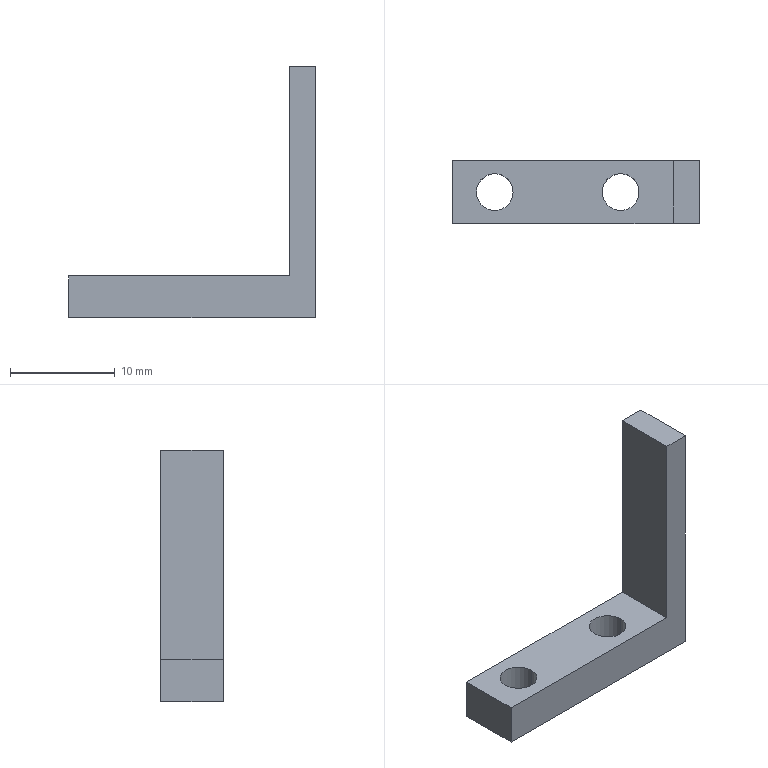Part | SolidWorks | features BaseBody 1 | 1 solid | 12 faces | box 23.5 x 6 x 24 mm | volume 787.031 mm3 | plane 8 | cylinder 4 | commonest cylinder face diameters 3.5 x4
STEP:
#1=CARTESIAN_POINT('',(-33.678,3.,0.));
#2=VERTEX_POINT('',#1);
#3=CARTESIAN_POINT('',(-37.178,3.,0.));
#4=VERTEX_POINT('',#3);
#5=CARTESIAN_POINT('',(-35.428,3.,0.));
#6=DIRECTION('',(0.,0.,-1.));
#7=DIRECTION('',(1.,0.,0.));
#8=AXIS2_PLACEMENT_3D('',#5,#6,#7);
#9=CIRCLE('',#8,1.75);
#10=EDGE_CURVE('',#2,#4,#9,.T.);
#11=ORIENTED_EDGE('',*,*,#10,.T.);
#12=CARTESIAN_POINT('',(-37.178,3.,4.));
#13=VERTEX_POINT('',#12);
#14=CARTESIAN_POINT('',(-37.178,3.,-30.121));
#15=DIRECTION('',(0.,0.,1.));
#16=VECTOR('',#15,1000.);
#17=LINE('',#14,#16);
#18=EDGE_CURVE('',#4,#13,#17,.T.);
#19=ORIENTED_EDGE('',*,*,#18,.T.);
#20=CARTESIAN_POINT('',(-33.678,3.,4.));
#21=VERTEX_POINT('',#20);
#22=CARTESIAN_POINT('',(-35.428,3.,4.));
#23=DIRECTION('',(0.,0.,-1.));
#24=DIRECTION('',(1.,0.,0.));
#25=AXIS2_PLACEMENT_3D('',#22,#23,#24);
#26=CIRCLE('',#25,1.75);
#27=EDGE_CURVE('',#21,#13,#26,.T.);
#28=ORIENTED_EDGE('',*,*,#27,.F.);
#29=CARTESIAN_POINT('',(-33.678,3.,-30.121));
#30=DIRECTION('',(0.,0.,1.));
#31=VECTOR('',#30,1000.);
#32=LINE('',#29,#31);
#33=EDGE_CURVE('',#2,#21,#32,.T.);
#34=ORIENTED_EDGE('',*,*,#33,.F.);
#35=EDGE_LOOP('',(#11,#19,#28,#34));
#36=FACE_OUTER_BOUND('',#35,.T.);
#37=CARTESIAN_POINT('',(-35.428,3.,-30.121));
#38=DIRECTION('',(0.,0.,1.));
#39=DIRECTION('',(1.,0.,0.));
#40=AXIS2_PLACEMENT_3D('',#37,#38,#39);
#41=CYLINDRICAL_SURFACE('',#40,1.75);
#42=ADVANCED_FACE('',(#36),#41,.F.);
#43=CARTESIAN_POINT('',(-21.678,3.,0.));
#44=VERTEX_POINT('',#43);
#45=CARTESIAN_POINT('',(-25.178,3.,0.));
#46=VERTEX_POINT('',#45);
#47=CARTESIAN_POINT('',(-23.428,3.,0.));
#48=DIRECTION('',(0.,0.,-1.));
#49=DIRECTION('',(1.,0.,0.));
#50=AXIS2_PLACEMENT_3D('',#47,#48,#49);
#51=CIRCLE('',#50,1.75);
#52=EDGE_CURVE('',#44,#46,#51,.T.);
#53=ORIENTED_EDGE('',*,*,#52,.T.);
#54=CARTESIAN_POINT('',(-25.178,3.,4.));
#55=VERTEX_POINT('',#54);
#56=CARTESIAN_POINT('',(-25.178,3.,-30.121));
#57=DIRECTION('',(0.,0.,1.));
#58=VECTOR('',#57,1000.);
#59=LINE('',#56,#58);
#60=EDGE_CURVE('',#46,#55,#59,.T.);
#61=ORIENTED_EDGE('',*,*,#60,.T.);
#62=CARTESIAN_POINT('',(-21.678,3.,4.));
#63=VERTEX_POINT('',#62);
#64=CARTESIAN_POINT('',(-23.428,3.,4.));
#65=DIRECTION('',(0.,0.,-1.));
#66=DIRECTION('',(1.,0.,0.));
#67=AXIS2_PLACEMENT_3D('',#64,#65,#66);
#68=CIRCLE('',#67,1.75);
#69=EDGE_CURVE('',#63,#55,#68,.T.);
#70=ORIENTED_EDGE('',*,*,#69,.F.);
#71=CARTESIAN_POINT('',(-21.678,3.,-30.121));
#72=DIRECTION('',(0.,0.,1.));
#73=VECTOR('',#72,1000.);
#74=LINE('',#71,#73);
#75=EDGE_CURVE('',#44,#63,#74,.T.);
#76=ORIENTED_EDGE('',*,*,#75,.F.);
#77=EDGE_LOOP('',(#53,#61,#70,#76));
#78=FACE_OUTER_BOUND('',#77,.T.);
#79=CARTESIAN_POINT('',(-23.428,3.,-30.121));
#80=DIRECTION('',(0.,0.,1.));
#81=DIRECTION('',(1.,0.,0.));
#82=AXIS2_PLACEMENT_3D('',#79,#80,#81);
#83=CYLINDRICAL_SURFACE('',#82,1.75);
#84=ADVANCED_FACE('',(#78),#83,.F.);
#85=CARTESIAN_POINT('',(-15.928,6.,0.));
#86=VERTEX_POINT('',#85);
#87=CARTESIAN_POINT('',(-15.928,6.,24.));
#88=VERTEX_POINT('',#87);
#89=CARTESIAN_POINT('',(-15.928,6.,0.));
#90=DIRECTION('',(0.,0.,1.));
#91=VECTOR('',#90,1000.);
#92=LINE('',#89,#91);
#93=EDGE_CURVE('',#86,#88,#92,.T.);
#94=ORIENTED_EDGE('',*,*,#93,.T.);
#95=CARTESIAN_POINT('',(-15.928,0.,24.));
#96=VERTEX_POINT('',#95);
#97=CARTESIAN_POINT('',(-15.928,6.,24.));
#98=DIRECTION('',(0.,-1.,0.));
#99=VECTOR('',#98,1000.);
#100=LINE('',#97,#99);
#101=EDGE_CURVE('',#88,#96,#100,.T.);
#102=ORIENTED_EDGE('',*,*,#101,.T.);
#103=CARTESIAN_POINT('',(-15.928,0.,0.));
#104=VERTEX_POINT('',#103);
#105=CARTESIAN_POINT('',(-15.928,0.,0.));
#106=DIRECTION('',(0.,0.,-1.));
#107=VECTOR('',#106,1000.);
#108=LINE('',#105,#107);
#109=EDGE_CURVE('',#96,#104,#108,.T.);
#110=ORIENTED_EDGE('',*,*,#109,.T.);
#111=CARTESIAN_POINT('',(-15.928,6.,0.));
#112=DIRECTION('',(0.,1.,0.));
#113=VECTOR('',#112,1000.);
#114=LINE('',#111,#113);
#115=EDGE_CURVE('',#104,#86,#114,.T.);
#116=ORIENTED_EDGE('',*,*,#115,.T.);
#117=EDGE_LOOP('',(#94,#102,#110,#116));
#118=FACE_OUTER_BOUND('',#117,.T.);
#119=CARTESIAN_POINT('',(-15.928,6.,0.));
#120=DIRECTION('',(1.,0.,0.));
#121=DIRECTION('',(0.,0.,-1.));
#122=AXIS2_PLACEMENT_3D('',#119,#120,#121);
#123=PLANE('',#122);
#124=ADVANCED_FACE('',(#118),#123,.T.);
#125=ORIENTED_EDGE('',*,*,#101,.F.);
#126=CARTESIAN_POINT('',(-18.428,6.,24.));
#127=VERTEX_POINT('',#126);
#128=CARTESIAN_POINT('',(-17.178,6.,24.));
#129=DIRECTION('',(-1.,0.,0.));
#130=VECTOR('',#129,1000.);
#131=LINE('',#128,#130);
#132=EDGE_CURVE('',#88,#127,#131,.T.);
#133=ORIENTED_EDGE('',*,*,#132,.T.);
#134=CARTESIAN_POINT('',(-18.428,0.,24.));
#135=VERTEX_POINT('',#134);
#136=CARTESIAN_POINT('',(-18.428,3.,24.));
#137=DIRECTION('',(0.,-1.,0.));
#138=VECTOR('',#137,1000.);
#139=LINE('',#136,#138);
#140=EDGE_CURVE('',#127,#135,#139,.T.);
#141=ORIENTED_EDGE('',*,*,#140,.T.);
#142=CARTESIAN_POINT('',(-17.178,0.,24.));
#143=DIRECTION('',(1.,0.,0.));
#144=VECTOR('',#143,1000.);
#145=LINE('',#142,#144);
#146=EDGE_CURVE('',#135,#96,#145,.T.);
#147=ORIENTED_EDGE('',*,*,#146,.T.);
#148=EDGE_LOOP('',(#125,#133,#141,#147));
#149=FACE_OUTER_BOUND('',#148,.T.);
#150=CARTESIAN_POINT('',(-17.178,3.,24.));
#151=DIRECTION('',(0.,0.,1.));
#152=DIRECTION('',(1.,0.,0.));
#153=AXIS2_PLACEMENT_3D('',#150,#151,#152);
#154=PLANE('',#153);
#155=ADVANCED_FACE('',(#149),#154,.T.);
#156=CARTESIAN_POINT('',(-39.428,6.,0.));
#157=VERTEX_POINT('',#156);
#158=CARTESIAN_POINT('',(-39.428,6.,0.));
#159=DIRECTION('',(-1.,0.,0.));
#160=VECTOR('',#159,1000.);
#161=LINE('',#158,#160);
#162=EDGE_CURVE('',#86,#157,#161,.T.);
#163=ORIENTED_EDGE('',*,*,#162,.T.);
#164=CARTESIAN_POINT('',(-39.428,6.,4.));
#165=VERTEX_POINT('',#164);
#166=CARTESIAN_POINT('',(-39.428,6.,0.));
#167=DIRECTION('',(0.,0.,1.));
#168=VECTOR('',#167,1000.);
#169=LINE('',#166,#168);
#170=EDGE_CURVE('',#157,#165,#169,.T.);
#171=ORIENTED_EDGE('',*,*,#170,.T.);
#172=CARTESIAN_POINT('',(-18.428,6.,4.));
#173=VERTEX_POINT('',#172);
#174=CARTESIAN_POINT('',(-39.428,6.,4.));
#175=DIRECTION('',(1.,0.,0.));
#176=VECTOR('',#175,1000.);
#177=LINE('',#174,#176);
#178=EDGE_CURVE('',#165,#173,#177,.T.);
#179=ORIENTED_EDGE('',*,*,#178,.T.);
#180=CARTESIAN_POINT('',(-18.428,6.,0.));
#181=DIRECTION('',(0.,0.,1.));
#182=VECTOR('',#181,1000.);
#183=LINE('',#180,#182);
#184=EDGE_CURVE('',#173,#127,#183,.T.);
#185=ORIENTED_EDGE('',*,*,#184,.T.);
#186=ORIENTED_EDGE('',*,*,#132,.F.);
#187=ORIENTED_EDGE('',*,*,#93,.F.);
#188=EDGE_LOOP('',(#163,#171,#179,#185,#186,#187));
#189=FACE_OUTER_BOUND('',#188,.T.);
#190=CARTESIAN_POINT('',(-39.428,6.,0.));
#191=DIRECTION('',(0.,1.,0.));
#192=DIRECTION('',(0.,0.,1.));
#193=AXIS2_PLACEMENT_3D('',#190,#191,#192);
#194=PLANE('',#193);
#195=ADVANCED_FACE('',(#189),#194,.T.);
#196=ORIENTED_EDGE('',*,*,#10,.F.);
#197=CARTESIAN_POINT('',(-35.428,3.,0.));
#198=DIRECTION('',(0.,0.,-1.));
#199=DIRECTION('',(1.,0.,0.));
#200=AXIS2_PLACEMENT_3D('',#197,#198,#199);
#201=CIRCLE('',#200,1.75);
#202=EDGE_CURVE('',#4,#2,#201,.T.);
#203=ORIENTED_EDGE('',*,*,#202,.F.);
#204=EDGE_LOOP('',(#196,#203));
#205=FACE_BOUND('',#204,.T.);
#206=ORIENTED_EDGE('',*,*,#52,.F.);
#207=CARTESIAN_POINT('',(-23.428,3.,0.));
#208=DIRECTION('',(0.,0.,-1.));
#209=DIRECTION('',(1.,0.,0.));
#210=AXIS2_PLACEMENT_3D('',#207,#208,#209);
#211=CIRCLE('',#210,1.75);
#212=EDGE_CURVE('',#46,#44,#211,.T.);
#213=ORIENTED_EDGE('',*,*,#212,.F.);
#214=EDGE_LOOP('',(#206,#213));
#215=FACE_BOUND('',#214,.T.);
#216=CARTESIAN_POINT('',(-39.428,0.,0.));
#217=VERTEX_POINT('',#216);
#218=CARTESIAN_POINT('',(-39.428,3.,0.));
#219=DIRECTION('',(0.,-1.,0.));
#220=VECTOR('',#219,1000.);
#221=LINE('',#218,#220);
#222=EDGE_CURVE('',#157,#217,#221,.T.);
#223=ORIENTED_EDGE('',*,*,#222,.F.);
#224=ORIENTED_EDGE('',*,*,#162,.F.);
#225=ORIENTED_EDGE('',*,*,#115,.F.);
#226=CARTESIAN_POINT('',(-27.678,0.,0.));
#227=DIRECTION('',(1.,0.,0.));
#228=VECTOR('',#227,1000.);
#229=LINE('',#226,#228);
#230=EDGE_CURVE('',#217,#104,#229,.T.);
#231=ORIENTED_EDGE('',*,*,#230,.F.);
#232=EDGE_LOOP('',(#223,#224,#225,#231));
#233=FACE_OUTER_BOUND('',#232,.T.);
#234=CARTESIAN_POINT('',(-27.678,3.,0.));
#235=DIRECTION('',(0.,0.,1.));
#236=DIRECTION('',(1.,0.,0.));
#237=AXIS2_PLACEMENT_3D('',#234,#235,#236);
#238=PLANE('',#237);
#239=ADVANCED_FACE('',(#205,#215,#233),#238,.F.);
#240=ORIENTED_EDGE('',*,*,#146,.F.);
#241=CARTESIAN_POINT('',(-18.428,0.,4.));
#242=VERTEX_POINT('',#241);
#243=CARTESIAN_POINT('',(-18.428,0.,0.));
#244=DIRECTION('',(0.,0.,-1.));
#245=VECTOR('',#244,1000.);
#246=LINE('',#243,#245);
#247=EDGE_CURVE('',#135,#242,#246,.T.);
#248=ORIENTED_EDGE('',*,*,#247,.T.);
#249=CARTESIAN_POINT('',(-39.428,0.,4.));
#250=VERTEX_POINT('',#249);
#251=CARTESIAN_POINT('',(-15.928,0.,4.));
#252=DIRECTION('',(-1.,0.,0.));
#253=VECTOR('',#252,1000.);
#254=LINE('',#251,#253);
#255=EDGE_CURVE('',#242,#250,#254,.T.);
#256=ORIENTED_EDGE('',*,*,#255,.T.);
#257=CARTESIAN_POINT('',(-39.428,0.,0.));
#258=DIRECTION('',(0.,0.,-1.));
#259=VECTOR('',#258,1000.);
#260=LINE('',#257,#259);
#261=EDGE_CURVE('',#250,#217,#260,.T.);
#262=ORIENTED_EDGE('',*,*,#261,.T.);
#263=ORIENTED_EDGE('',*,*,#230,.T.);
#264=ORIENTED_EDGE('',*,*,#109,.F.);
#265=EDGE_LOOP('',(#240,#248,#256,#262,#263,#264));
#266=FACE_OUTER_BOUND('',#265,.T.);
#267=CARTESIAN_POINT('',(-15.928,0.,0.));
#268=DIRECTION('',(0.,-1.,0.));
#269=DIRECTION('',(0.,0.,-1.));
#270=AXIS2_PLACEMENT_3D('',#267,#268,#269);
#271=PLANE('',#270);
#272=ADVANCED_FACE('',(#266),#271,.T.);
#273=CARTESIAN_POINT('',(-18.428,0.,4.));
#274=DIRECTION('',(0.,-1.,0.));
#275=VECTOR('',#274,1000.);
#276=LINE('',#273,#275);
#277=EDGE_CURVE('',#173,#242,#276,.T.);
#278=ORIENTED_EDGE('',*,*,#277,.T.);
#279=ORIENTED_EDGE('',*,*,#247,.F.);
#280=ORIENTED_EDGE('',*,*,#140,.F.);
#281=ORIENTED_EDGE('',*,*,#184,.F.);
#282=EDGE_LOOP('',(#278,#279,#280,#281));
#283=FACE_OUTER_BOUND('',#282,.T.);
#284=CARTESIAN_POINT('',(-18.428,0.,4.));
#285=DIRECTION('',(-1.,0.,0.));
#286=DIRECTION('',(0.,0.,1.));
#287=AXIS2_PLACEMENT_3D('',#284,#285,#286);
#288=PLANE('',#287);
#289=ADVANCED_FACE('',(#283),#288,.T.);
#290=ORIENTED_EDGE('',*,*,#222,.T.);
#291=ORIENTED_EDGE('',*,*,#261,.F.);
#292=CARTESIAN_POINT('',(-39.428,0.,4.));
#293=DIRECTION('',(0.,1.,0.));
#294=VECTOR('',#293,1000.);
#295=LINE('',#292,#294);
#296=EDGE_CURVE('',#250,#165,#295,.T.);
#297=ORIENTED_EDGE('',*,*,#296,.T.);
#298=ORIENTED_EDGE('',*,*,#170,.F.);
#299=EDGE_LOOP('',(#290,#291,#297,#298));
#300=FACE_OUTER_BOUND('',#299,.T.);
#301=CARTESIAN_POINT('',(-39.428,0.,0.));
#302=DIRECTION('',(-1.,0.,0.));
#303=DIRECTION('',(0.,0.,1.));
#304=AXIS2_PLACEMENT_3D('',#301,#302,#303);
#305=PLANE('',#304);
#306=ADVANCED_FACE('',(#300),#305,.T.);
#307=ORIENTED_EDGE('',*,*,#27,.T.);
#308=CARTESIAN_POINT('',(-35.428,3.,4.));
#309=DIRECTION('',(0.,0.,-1.));
#310=DIRECTION('',(1.,0.,0.));
#311=AXIS2_PLACEMENT_3D('',#308,#309,#310);
#312=CIRCLE('',#311,1.75);
#313=EDGE_CURVE('',#13,#21,#312,.T.);
#314=ORIENTED_EDGE('',*,*,#313,.T.);
#315=EDGE_LOOP('',(#307,#314));
#316=FACE_BOUND('',#315,.T.);
#317=ORIENTED_EDGE('',*,*,#69,.T.);
#318=CARTESIAN_POINT('',(-23.428,3.,4.));
#319=DIRECTION('',(0.,0.,-1.));
#320=DIRECTION('',(1.,0.,0.));
#321=AXIS2_PLACEMENT_3D('',#318,#319,#320);
#322=CIRCLE('',#321,1.75);
#323=EDGE_CURVE('',#55,#63,#322,.T.);
#324=ORIENTED_EDGE('',*,*,#323,.T.);
#325=EDGE_LOOP('',(#317,#324));
#326=FACE_BOUND('',#325,.T.);
#327=ORIENTED_EDGE('',*,*,#296,.F.);
#328=ORIENTED_EDGE('',*,*,#255,.F.);
#329=ORIENTED_EDGE('',*,*,#277,.F.);
#330=ORIENTED_EDGE('',*,*,#178,.F.);
#331=EDGE_LOOP('',(#327,#328,#329,#330));
#332=FACE_OUTER_BOUND('',#331,.T.);
#333=CARTESIAN_POINT('',(-27.678,3.,4.));
#334=DIRECTION('',(0.,0.,1.));
#335=DIRECTION('',(1.,0.,0.));
#336=AXIS2_PLACEMENT_3D('',#333,#334,#335);
#337=PLANE('',#336);
#338=ADVANCED_FACE('',(#316,#326,#332),#337,.T.);
#339=ORIENTED_EDGE('',*,*,#18,.F.);
#340=ORIENTED_EDGE('',*,*,#202,.T.);
#341=ORIENTED_EDGE('',*,*,#33,.T.);
#342=ORIENTED_EDGE('',*,*,#313,.F.);
#343=EDGE_LOOP('',(#339,#340,#341,#342));
#344=FACE_OUTER_BOUND('',#343,.T.);
#345=CARTESIAN_POINT('',(-35.428,3.,-30.121));
#346=DIRECTION('',(0.,0.,1.));
#347=DIRECTION('',(1.,0.,0.));
#348=AXIS2_PLACEMENT_3D('',#345,#346,#347);
#349=CYLINDRICAL_SURFACE('',#348,1.75);
#350=ADVANCED_FACE('',(#344),#349,.F.);
#351=ORIENTED_EDGE('',*,*,#60,.F.);
#352=ORIENTED_EDGE('',*,*,#212,.T.);
#353=ORIENTED_EDGE('',*,*,#75,.T.);
#354=ORIENTED_EDGE('',*,*,#323,.F.);
#355=EDGE_LOOP('',(#351,#352,#353,#354));
#356=FACE_OUTER_BOUND('',#355,.T.);
#357=CARTESIAN_POINT('',(-23.428,3.,-30.121));
#358=DIRECTION('',(0.,0.,1.));
#359=DIRECTION('',(1.,0.,0.));
#360=AXIS2_PLACEMENT_3D('',#357,#358,#359);
#361=CYLINDRICAL_SURFACE('',#360,1.75);
#362=ADVANCED_FACE('',(#356),#361,.F.);
#363=CLOSED_SHELL('',(#42,#84,#124,#155,#195,#239,#272,#289,#306,#338,#350,#362));
#364=MANIFOLD_SOLID_BREP('',#363);
#365=CARTESIAN_POINT('',(0.,0.,0.));
#366=DIRECTION('',(0.,0.,1.));
#367=DIRECTION('',(1.,0.,0.));
#368=AXIS2_PLACEMENT_3D('',#365,#366,#367);
#369=(LENGTH_UNIT()NAMED_UNIT(*)SI_UNIT(.MILLI.,.METRE.));
#370=UNCERTAINTY_MEASURE_WITH_UNIT(LENGTH_MEASURE(0.00001),#369,'','');
#371=(NAMED_UNIT(*)PLANE_ANGLE_UNIT()SI_UNIT($,.RADIAN.));
#372=(NAMED_UNIT(*)SI_UNIT($,.STERADIAN.)SOLID_ANGLE_UNIT());
#373=(GEOMETRIC_REPRESENTATION_CONTEXT(3)GLOBAL_UNCERTAINTY_ASSIGNED_CONTEXT((#370))GLOBAL_UNIT_ASSIGNED_CONTEXT((#369,#371,#372))REPRESENTATION_CONTEXT('',''));
#374=ADVANCED_BREP_SHAPE_REPRESENTATION('',(#364,#368),#373);